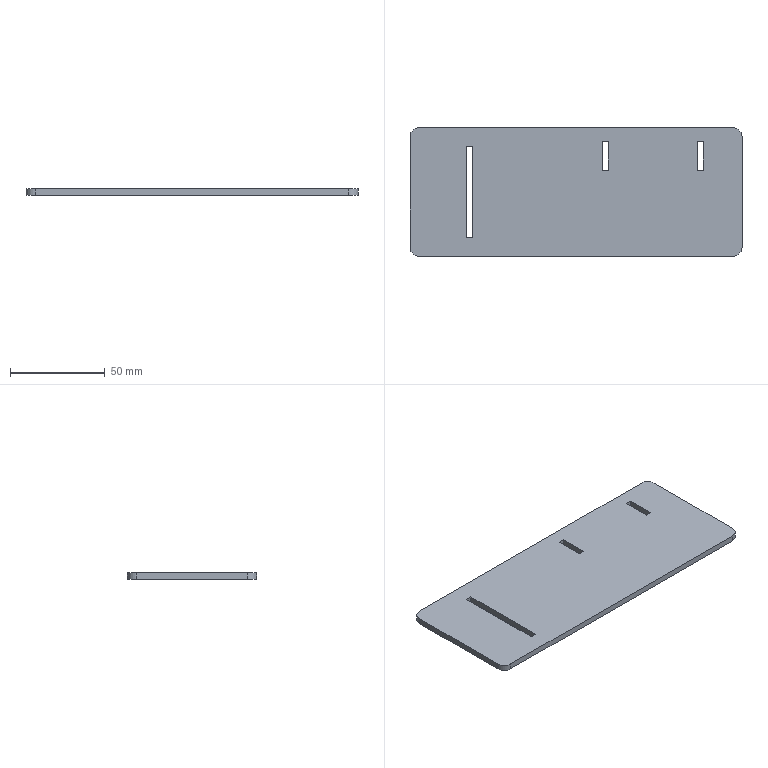Part | SolidWorks | features FlatPattern 1, SMBaseFlange 1, SheetMetal 1 | 1 solid | 22 faces | box 175 x 68 x 3.2 mm | volume 37213 mm3 | plane 18 | cylinder 4 | commonest cylinder face diameters 10 x4
STEP:
#1=CARTESIAN_POINT('',(-211.3,93.,3.2));
#2=VERTEX_POINT('',#1);
#3=CARTESIAN_POINT('',(-211.3,108.,3.2));
#4=VERTEX_POINT('',#3);
#5=CARTESIAN_POINT('',(-211.3,108.,3.2));
#6=DIRECTION('',(0.,1.,0.));
#7=VECTOR('',#6,1000.);
#8=LINE('',#5,#7);
#9=EDGE_CURVE('',#2,#4,#8,.T.);
#10=ORIENTED_EDGE('',*,*,#9,.F.);
#11=CARTESIAN_POINT('',(-214.5,93.,3.2));
#12=VERTEX_POINT('',#11);
#13=CARTESIAN_POINT('',(-211.3,93.,3.2));
#14=DIRECTION('',(1.,0.,0.));
#15=VECTOR('',#14,1000.);
#16=LINE('',#13,#15);
#17=EDGE_CURVE('',#12,#2,#16,.T.);
#18=ORIENTED_EDGE('',*,*,#17,.F.);
#19=CARTESIAN_POINT('',(-214.5,108.,3.2));
#20=VERTEX_POINT('',#19);
#21=CARTESIAN_POINT('',(-214.5,108.,3.2));
#22=DIRECTION('',(0.,-1.,0.));
#23=VECTOR('',#22,1000.);
#24=LINE('',#21,#23);
#25=EDGE_CURVE('',#20,#12,#24,.T.);
#26=ORIENTED_EDGE('',*,*,#25,.F.);
#27=CARTESIAN_POINT('',(-211.3,108.,3.2));
#28=DIRECTION('',(-1.,0.,0.));
#29=VECTOR('',#28,1000.);
#30=LINE('',#27,#29);
#31=EDGE_CURVE('',#4,#20,#30,.T.);
#32=ORIENTED_EDGE('',*,*,#31,.F.);
#33=EDGE_LOOP('',(#10,#18,#26,#32));
#34=FACE_BOUND('',#33,.T.);
#35=CARTESIAN_POINT('',(-190.9,110.5,3.2));
#36=VERTEX_POINT('',#35);
#37=CARTESIAN_POINT('',(-195.9,115.5,3.2));
#38=VERTEX_POINT('',#37);
#39=CARTESIAN_POINT('',(-195.9,110.5,3.2));
#40=DIRECTION('',(0.,0.,1.));
#41=DIRECTION('',(-1.,0.,0.));
#42=AXIS2_PLACEMENT_3D('',#39,#40,#41);
#43=CIRCLE('',#42,5.);
#44=EDGE_CURVE('',#36,#38,#43,.T.);
#45=ORIENTED_EDGE('',*,*,#44,.T.);
#46=CARTESIAN_POINT('',(-360.9,115.5,3.2));
#47=VERTEX_POINT('',#46);
#48=CARTESIAN_POINT('',(-360.9,115.5,3.2));
#49=DIRECTION('',(-1.,0.,0.));
#50=VECTOR('',#49,1000.);
#51=LINE('',#48,#50);
#52=EDGE_CURVE('',#38,#47,#51,.T.);
#53=ORIENTED_EDGE('',*,*,#52,.T.);
#54=CARTESIAN_POINT('',(-365.9,110.5,3.2));
#55=VERTEX_POINT('',#54);
#56=CARTESIAN_POINT('',(-360.9,110.5,3.2));
#57=DIRECTION('',(0.,0.,1.));
#58=DIRECTION('',(-1.,0.,0.));
#59=AXIS2_PLACEMENT_3D('',#56,#57,#58);
#60=CIRCLE('',#59,5.);
#61=EDGE_CURVE('',#47,#55,#60,.T.);
#62=ORIENTED_EDGE('',*,*,#61,.T.);
#63=CARTESIAN_POINT('',(-365.9,52.5,3.2));
#64=VERTEX_POINT('',#63);
#65=CARTESIAN_POINT('',(-365.9,52.5,3.2));
#66=DIRECTION('',(0.,-1.,0.));
#67=VECTOR('',#66,1000.);
#68=LINE('',#65,#67);
#69=EDGE_CURVE('',#55,#64,#68,.T.);
#70=ORIENTED_EDGE('',*,*,#69,.T.);
#71=CARTESIAN_POINT('',(-360.9,47.5,3.2));
#72=VERTEX_POINT('',#71);
#73=CARTESIAN_POINT('',(-360.9,52.5,3.2));
#74=DIRECTION('',(0.,0.,1.));
#75=DIRECTION('',(-1.,0.,0.));
#76=AXIS2_PLACEMENT_3D('',#73,#74,#75);
#77=CIRCLE('',#76,5.);
#78=EDGE_CURVE('',#64,#72,#77,.T.);
#79=ORIENTED_EDGE('',*,*,#78,.T.);
#80=CARTESIAN_POINT('',(-195.9,47.5,3.2));
#81=VERTEX_POINT('',#80);
#82=CARTESIAN_POINT('',(-360.9,47.5,3.2));
#83=DIRECTION('',(1.,0.,0.));
#84=VECTOR('',#83,1000.);
#85=LINE('',#82,#84);
#86=EDGE_CURVE('',#72,#81,#85,.T.);
#87=ORIENTED_EDGE('',*,*,#86,.T.);
#88=CARTESIAN_POINT('',(-190.9,52.5,3.2));
#89=VERTEX_POINT('',#88);
#90=CARTESIAN_POINT('',(-195.9,52.5,3.2));
#91=DIRECTION('',(0.,0.,1.));
#92=DIRECTION('',(1.,0.,0.));
#93=AXIS2_PLACEMENT_3D('',#90,#91,#92);
#94=CIRCLE('',#93,5.);
#95=EDGE_CURVE('',#81,#89,#94,.T.);
#96=ORIENTED_EDGE('',*,*,#95,.T.);
#97=CARTESIAN_POINT('',(-190.9,52.5,3.2));
#98=DIRECTION('',(0.,1.,0.));
#99=VECTOR('',#98,1000.);
#100=LINE('',#97,#99);
#101=EDGE_CURVE('',#89,#36,#100,.T.);
#102=ORIENTED_EDGE('',*,*,#101,.T.);
#103=EDGE_LOOP('',(#45,#53,#62,#70,#79,#87,#96,#102));
#104=FACE_OUTER_BOUND('',#103,.T.);
#105=CARTESIAN_POINT('',(-335.9,105.5,3.2));
#106=VERTEX_POINT('',#105);
#107=CARTESIAN_POINT('',(-335.9,57.5,3.2));
#108=VERTEX_POINT('',#107);
#109=CARTESIAN_POINT('',(-335.9,105.5,3.2));
#110=DIRECTION('',(0.,-1.,0.));
#111=VECTOR('',#110,1000.);
#112=LINE('',#109,#111);
#113=EDGE_CURVE('',#106,#108,#112,.T.);
#114=ORIENTED_EDGE('',*,*,#113,.F.);
#115=CARTESIAN_POINT('',(-332.7,105.5,3.2));
#116=VERTEX_POINT('',#115);
#117=CARTESIAN_POINT('',(-335.9,105.5,3.2));
#118=DIRECTION('',(-1.,0.,0.));
#119=VECTOR('',#118,1000.);
#120=LINE('',#117,#119);
#121=EDGE_CURVE('',#116,#106,#120,.T.);
#122=ORIENTED_EDGE('',*,*,#121,.F.);
#123=CARTESIAN_POINT('',(-332.7,57.5,3.2));
#124=VERTEX_POINT('',#123);
#125=CARTESIAN_POINT('',(-332.7,105.5,3.2));
#126=DIRECTION('',(0.,1.,0.));
#127=VECTOR('',#126,1000.);
#128=LINE('',#125,#127);
#129=EDGE_CURVE('',#124,#116,#128,.T.);
#130=ORIENTED_EDGE('',*,*,#129,.F.);
#131=CARTESIAN_POINT('',(-335.9,57.5,3.2));
#132=DIRECTION('',(1.,0.,0.));
#133=VECTOR('',#132,1000.);
#134=LINE('',#131,#133);
#135=EDGE_CURVE('',#108,#124,#134,.T.);
#136=ORIENTED_EDGE('',*,*,#135,.F.);
#137=EDGE_LOOP('',(#114,#122,#130,#136));
#138=FACE_BOUND('',#137,.T.);
#139=CARTESIAN_POINT('',(-261.3,93.,3.2));
#140=VERTEX_POINT('',#139);
#141=CARTESIAN_POINT('',(-261.3,108.,3.2));
#142=VERTEX_POINT('',#141);
#143=CARTESIAN_POINT('',(-261.3,108.,3.2));
#144=DIRECTION('',(0.,1.,0.));
#145=VECTOR('',#144,1000.);
#146=LINE('',#143,#145);
#147=EDGE_CURVE('',#140,#142,#146,.T.);
#148=ORIENTED_EDGE('',*,*,#147,.F.);
#149=CARTESIAN_POINT('',(-264.5,93.,3.2));
#150=VERTEX_POINT('',#149);
#151=CARTESIAN_POINT('',(-261.3,93.,3.2));
#152=DIRECTION('',(1.,0.,0.));
#153=VECTOR('',#152,1000.);
#154=LINE('',#151,#153);
#155=EDGE_CURVE('',#150,#140,#154,.T.);
#156=ORIENTED_EDGE('',*,*,#155,.F.);
#157=CARTESIAN_POINT('',(-264.5,108.,3.2));
#158=VERTEX_POINT('',#157);
#159=CARTESIAN_POINT('',(-264.5,108.,3.2));
#160=DIRECTION('',(0.,-1.,0.));
#161=VECTOR('',#160,1000.);
#162=LINE('',#159,#161);
#163=EDGE_CURVE('',#158,#150,#162,.T.);
#164=ORIENTED_EDGE('',*,*,#163,.F.);
#165=CARTESIAN_POINT('',(-261.3,108.,3.2));
#166=DIRECTION('',(-1.,0.,0.));
#167=VECTOR('',#166,1000.);
#168=LINE('',#165,#167);
#169=EDGE_CURVE('',#142,#158,#168,.T.);
#170=ORIENTED_EDGE('',*,*,#169,.F.);
#171=EDGE_LOOP('',(#148,#156,#164,#170));
#172=FACE_BOUND('',#171,.T.);
#173=CARTESIAN_POINT('',(-195.9,110.5,3.2));
#174=DIRECTION('',(0.,0.,-1.));
#175=DIRECTION('',(-1.,0.,0.));
#176=AXIS2_PLACEMENT_3D('',#173,#174,#175);
#177=PLANE('',#176);
#178=ADVANCED_FACE('',(#34,#104,#138,#172),#177,.F.);
#179=CARTESIAN_POINT('',(-190.9,110.5,0.));
#180=VERTEX_POINT('',#179);
#181=CARTESIAN_POINT('',(-195.9,115.5,0.));
#182=VERTEX_POINT('',#181);
#183=CARTESIAN_POINT('',(-195.9,110.5,0.));
#184=DIRECTION('',(0.,0.,1.));
#185=DIRECTION('',(-1.,0.,0.));
#186=AXIS2_PLACEMENT_3D('',#183,#184,#185);
#187=CIRCLE('',#186,5.);
#188=EDGE_CURVE('',#180,#182,#187,.T.);
#189=ORIENTED_EDGE('',*,*,#188,.F.);
#190=CARTESIAN_POINT('',(-190.9,52.5,0.));
#191=VERTEX_POINT('',#190);
#192=CARTESIAN_POINT('',(-190.9,52.5,0.));
#193=DIRECTION('',(0.,1.,0.));
#194=VECTOR('',#193,1000.);
#195=LINE('',#192,#194);
#196=EDGE_CURVE('',#191,#180,#195,.T.);
#197=ORIENTED_EDGE('',*,*,#196,.F.);
#198=CARTESIAN_POINT('',(-195.9,47.5,0.));
#199=VERTEX_POINT('',#198);
#200=CARTESIAN_POINT('',(-195.9,52.5,0.));
#201=DIRECTION('',(0.,0.,1.));
#202=DIRECTION('',(1.,0.,0.));
#203=AXIS2_PLACEMENT_3D('',#200,#201,#202);
#204=CIRCLE('',#203,5.);
#205=EDGE_CURVE('',#199,#191,#204,.T.);
#206=ORIENTED_EDGE('',*,*,#205,.F.);
#207=CARTESIAN_POINT('',(-360.9,47.5,0.));
#208=VERTEX_POINT('',#207);
#209=CARTESIAN_POINT('',(-360.9,47.5,0.));
#210=DIRECTION('',(1.,0.,0.));
#211=VECTOR('',#210,1000.);
#212=LINE('',#209,#211);
#213=EDGE_CURVE('',#208,#199,#212,.T.);
#214=ORIENTED_EDGE('',*,*,#213,.F.);
#215=CARTESIAN_POINT('',(-365.9,52.5,0.));
#216=VERTEX_POINT('',#215);
#217=CARTESIAN_POINT('',(-360.9,52.5,0.));
#218=DIRECTION('',(0.,0.,1.));
#219=DIRECTION('',(-1.,0.,0.));
#220=AXIS2_PLACEMENT_3D('',#217,#218,#219);
#221=CIRCLE('',#220,5.);
#222=EDGE_CURVE('',#216,#208,#221,.T.);
#223=ORIENTED_EDGE('',*,*,#222,.F.);
#224=CARTESIAN_POINT('',(-365.9,110.5,0.));
#225=VERTEX_POINT('',#224);
#226=CARTESIAN_POINT('',(-365.9,52.5,0.));
#227=DIRECTION('',(0.,-1.,0.));
#228=VECTOR('',#227,1000.);
#229=LINE('',#226,#228);
#230=EDGE_CURVE('',#225,#216,#229,.T.);
#231=ORIENTED_EDGE('',*,*,#230,.F.);
#232=CARTESIAN_POINT('',(-360.9,115.5,0.));
#233=VERTEX_POINT('',#232);
#234=CARTESIAN_POINT('',(-360.9,110.5,0.));
#235=DIRECTION('',(0.,0.,1.));
#236=DIRECTION('',(-1.,0.,0.));
#237=AXIS2_PLACEMENT_3D('',#234,#235,#236);
#238=CIRCLE('',#237,5.);
#239=EDGE_CURVE('',#233,#225,#238,.T.);
#240=ORIENTED_EDGE('',*,*,#239,.F.);
#241=CARTESIAN_POINT('',(-360.9,115.5,0.));
#242=DIRECTION('',(-1.,0.,0.));
#243=VECTOR('',#242,1000.);
#244=LINE('',#241,#243);
#245=EDGE_CURVE('',#182,#233,#244,.T.);
#246=ORIENTED_EDGE('',*,*,#245,.F.);
#247=EDGE_LOOP('',(#189,#197,#206,#214,#223,#231,#240,#246));
#248=FACE_OUTER_BOUND('',#247,.T.);
#249=CARTESIAN_POINT('',(-332.7,105.5,0.));
#250=VERTEX_POINT('',#249);
#251=CARTESIAN_POINT('',(-335.9,105.5,0.));
#252=VERTEX_POINT('',#251);
#253=CARTESIAN_POINT('',(-335.9,105.5,0.));
#254=DIRECTION('',(-1.,0.,0.));
#255=VECTOR('',#254,1000.);
#256=LINE('',#253,#255);
#257=EDGE_CURVE('',#250,#252,#256,.T.);
#258=ORIENTED_EDGE('',*,*,#257,.T.);
#259=CARTESIAN_POINT('',(-335.9,57.5,0.));
#260=VERTEX_POINT('',#259);
#261=CARTESIAN_POINT('',(-335.9,105.5,0.));
#262=DIRECTION('',(0.,-1.,0.));
#263=VECTOR('',#262,1000.);
#264=LINE('',#261,#263);
#265=EDGE_CURVE('',#252,#260,#264,.T.);
#266=ORIENTED_EDGE('',*,*,#265,.T.);
#267=CARTESIAN_POINT('',(-332.7,57.5,0.));
#268=VERTEX_POINT('',#267);
#269=CARTESIAN_POINT('',(-335.9,57.5,0.));
#270=DIRECTION('',(1.,0.,0.));
#271=VECTOR('',#270,1000.);
#272=LINE('',#269,#271);
#273=EDGE_CURVE('',#260,#268,#272,.T.);
#274=ORIENTED_EDGE('',*,*,#273,.T.);
#275=CARTESIAN_POINT('',(-332.7,105.5,0.));
#276=DIRECTION('',(0.,1.,0.));
#277=VECTOR('',#276,1000.);
#278=LINE('',#275,#277);
#279=EDGE_CURVE('',#268,#250,#278,.T.);
#280=ORIENTED_EDGE('',*,*,#279,.T.);
#281=EDGE_LOOP('',(#258,#266,#274,#280));
#282=FACE_BOUND('',#281,.T.);
#283=CARTESIAN_POINT('',(-214.5,93.,0.));
#284=VERTEX_POINT('',#283);
#285=CARTESIAN_POINT('',(-211.3,93.,0.));
#286=VERTEX_POINT('',#285);
#287=CARTESIAN_POINT('',(-211.3,93.,0.));
#288=DIRECTION('',(1.,0.,0.));
#289=VECTOR('',#288,1000.);
#290=LINE('',#287,#289);
#291=EDGE_CURVE('',#284,#286,#290,.T.);
#292=ORIENTED_EDGE('',*,*,#291,.T.);
#293=CARTESIAN_POINT('',(-211.3,108.,0.));
#294=VERTEX_POINT('',#293);
#295=CARTESIAN_POINT('',(-211.3,108.,0.));
#296=DIRECTION('',(0.,1.,0.));
#297=VECTOR('',#296,1000.);
#298=LINE('',#295,#297);
#299=EDGE_CURVE('',#286,#294,#298,.T.);
#300=ORIENTED_EDGE('',*,*,#299,.T.);
#301=CARTESIAN_POINT('',(-214.5,108.,0.));
#302=VERTEX_POINT('',#301);
#303=CARTESIAN_POINT('',(-211.3,108.,0.));
#304=DIRECTION('',(-1.,0.,0.));
#305=VECTOR('',#304,1000.);
#306=LINE('',#303,#305);
#307=EDGE_CURVE('',#294,#302,#306,.T.);
#308=ORIENTED_EDGE('',*,*,#307,.T.);
#309=CARTESIAN_POINT('',(-214.5,108.,0.));
#310=DIRECTION('',(0.,-1.,0.));
#311=VECTOR('',#310,1000.);
#312=LINE('',#309,#311);
#313=EDGE_CURVE('',#302,#284,#312,.T.);
#314=ORIENTED_EDGE('',*,*,#313,.T.);
#315=EDGE_LOOP('',(#292,#300,#308,#314));
#316=FACE_BOUND('',#315,.T.);
#317=CARTESIAN_POINT('',(-264.5,93.,0.));
#318=VERTEX_POINT('',#317);
#319=CARTESIAN_POINT('',(-261.3,93.,0.));
#320=VERTEX_POINT('',#319);
#321=CARTESIAN_POINT('',(-261.3,93.,0.));
#322=DIRECTION('',(1.,0.,0.));
#323=VECTOR('',#322,1000.);
#324=LINE('',#321,#323);
#325=EDGE_CURVE('',#318,#320,#324,.T.);
#326=ORIENTED_EDGE('',*,*,#325,.T.);
#327=CARTESIAN_POINT('',(-261.3,108.,0.));
#328=VERTEX_POINT('',#327);
#329=CARTESIAN_POINT('',(-261.3,108.,0.));
#330=DIRECTION('',(0.,1.,0.));
#331=VECTOR('',#330,1000.);
#332=LINE('',#329,#331);
#333=EDGE_CURVE('',#320,#328,#332,.T.);
#334=ORIENTED_EDGE('',*,*,#333,.T.);
#335=CARTESIAN_POINT('',(-264.5,108.,0.));
#336=VERTEX_POINT('',#335);
#337=CARTESIAN_POINT('',(-261.3,108.,0.));
#338=DIRECTION('',(-1.,0.,0.));
#339=VECTOR('',#338,1000.);
#340=LINE('',#337,#339);
#341=EDGE_CURVE('',#328,#336,#340,.T.);
#342=ORIENTED_EDGE('',*,*,#341,.T.);
#343=CARTESIAN_POINT('',(-264.5,108.,0.));
#344=DIRECTION('',(0.,-1.,0.));
#345=VECTOR('',#344,1000.);
#346=LINE('',#343,#345);
#347=EDGE_CURVE('',#336,#318,#346,.T.);
#348=ORIENTED_EDGE('',*,*,#347,.T.);
#349=EDGE_LOOP('',(#326,#334,#342,#348));
#350=FACE_BOUND('',#349,.T.);
#351=CARTESIAN_POINT('',(-195.9,110.5,0.));
#352=DIRECTION('',(0.,0.,-1.));
#353=DIRECTION('',(-1.,0.,0.));
#354=AXIS2_PLACEMENT_3D('',#351,#352,#353);
#355=PLANE('',#354);
#356=ADVANCED_FACE('',(#248,#282,#316,#350),#355,.T.);
#357=ORIENTED_EDGE('',*,*,#188,.T.);
#358=CARTESIAN_POINT('',(-195.9,115.5,3.2));
#359=DIRECTION('',(0.,0.,-1.));
#360=VECTOR('',#359,1000.);
#361=LINE('',#358,#360);
#362=EDGE_CURVE('',#38,#182,#361,.T.);
#363=ORIENTED_EDGE('',*,*,#362,.F.);
#364=ORIENTED_EDGE('',*,*,#44,.F.);
#365=CARTESIAN_POINT('',(-190.9,110.5,3.2));
#366=DIRECTION('',(0.,0.,-1.));
#367=VECTOR('',#366,1000.);
#368=LINE('',#365,#367);
#369=EDGE_CURVE('',#36,#180,#368,.T.);
#370=ORIENTED_EDGE('',*,*,#369,.T.);
#371=EDGE_LOOP('',(#357,#363,#364,#370));
#372=FACE_OUTER_BOUND('',#371,.T.);
#373=CARTESIAN_POINT('',(-195.9,110.5,3.2));
#374=DIRECTION('',(0.,0.,-1.));
#375=DIRECTION('',(-1.,0.,0.));
#376=AXIS2_PLACEMENT_3D('',#373,#374,#375);
#377=CYLINDRICAL_SURFACE('',#376,5.);
#378=ADVANCED_FACE('',(#372),#377,.T.);
#379=ORIENTED_EDGE('',*,*,#245,.T.);
#380=CARTESIAN_POINT('',(-360.9,115.5,3.2));
#381=DIRECTION('',(0.,0.,-1.));
#382=VECTOR('',#381,1000.);
#383=LINE('',#380,#382);
#384=EDGE_CURVE('',#47,#233,#383,.T.);
#385=ORIENTED_EDGE('',*,*,#384,.F.);
#386=ORIENTED_EDGE('',*,*,#52,.F.);
#387=ORIENTED_EDGE('',*,*,#362,.T.);
#388=EDGE_LOOP('',(#379,#385,#386,#387));
#389=FACE_OUTER_BOUND('',#388,.T.);
#390=CARTESIAN_POINT('',(-360.9,115.5,3.2));
#391=DIRECTION('',(0.,-1.,0.));
#392=DIRECTION('',(0.,0.,-1.));
#393=AXIS2_PLACEMENT_3D('',#390,#391,#392);
#394=PLANE('',#393);
#395=ADVANCED_FACE('',(#389),#394,.F.);
#396=ORIENTED_EDGE('',*,*,#239,.T.);
#397=CARTESIAN_POINT('',(-365.9,110.5,3.2));
#398=DIRECTION('',(0.,0.,-1.));
#399=VECTOR('',#398,1000.);
#400=LINE('',#397,#399);
#401=EDGE_CURVE('',#55,#225,#400,.T.);
#402=ORIENTED_EDGE('',*,*,#401,.F.);
#403=ORIENTED_EDGE('',*,*,#61,.F.);
#404=ORIENTED_EDGE('',*,*,#384,.T.);
#405=EDGE_LOOP('',(#396,#402,#403,#404));
#406=FACE_OUTER_BOUND('',#405,.T.);
#407=CARTESIAN_POINT('',(-360.9,110.5,3.2));
#408=DIRECTION('',(0.,0.,-1.));
#409=DIRECTION('',(-1.,0.,0.));
#410=AXIS2_PLACEMENT_3D('',#407,#408,#409);
#411=CYLINDRICAL_SURFACE('',#410,5.);
#412=ADVANCED_FACE('',(#406),#411,.T.);
#413=ORIENTED_EDGE('',*,*,#230,.T.);
#414=CARTESIAN_POINT('',(-365.9,52.5,3.2));
#415=DIRECTION('',(0.,0.,-1.));
#416=VECTOR('',#415,1000.);
#417=LINE('',#414,#416);
#418=EDGE_CURVE('',#64,#216,#417,.T.);
#419=ORIENTED_EDGE('',*,*,#418,.F.);
#420=ORIENTED_EDGE('',*,*,#69,.F.);
#421=ORIENTED_EDGE('',*,*,#401,.T.);
#422=EDGE_LOOP('',(#413,#419,#420,#421));
#423=FACE_OUTER_BOUND('',#422,.T.);
#424=CARTESIAN_POINT('',(-365.9,52.5,3.2));
#425=DIRECTION('',(1.,0.,0.));
#426=DIRECTION('',(0.,0.,-1.));
#427=AXIS2_PLACEMENT_3D('',#424,#425,#426);
#428=PLANE('',#427);
#429=ADVANCED_FACE('',(#423),#428,.F.);
#430=ORIENTED_EDGE('',*,*,#222,.T.);
#431=CARTESIAN_POINT('',(-360.9,47.5,3.2));
#432=DIRECTION('',(0.,0.,-1.));
#433=VECTOR('',#432,1000.);
#434=LINE('',#431,#433);
#435=EDGE_CURVE('',#72,#208,#434,.T.);
#436=ORIENTED_EDGE('',*,*,#435,.F.);
#437=ORIENTED_EDGE('',*,*,#78,.F.);
#438=ORIENTED_EDGE('',*,*,#418,.T.);
#439=EDGE_LOOP('',(#430,#436,#437,#438));
#440=FACE_OUTER_BOUND('',#439,.T.);
#441=CARTESIAN_POINT('',(-360.9,52.5,3.2));
#442=DIRECTION('',(0.,0.,-1.));
#443=DIRECTION('',(-1.,0.,0.));
#444=AXIS2_PLACEMENT_3D('',#441,#442,#443);
#445=CYLINDRICAL_SURFACE('',#444,5.);
#446=ADVANCED_FACE('',(#440),#445,.T.);
#447=ORIENTED_EDGE('',*,*,#213,.T.);
#448=CARTESIAN_POINT('',(-195.9,47.5,3.2));
#449=DIRECTION('',(0.,0.,-1.));
#450=VECTOR('',#449,1000.);
#451=LINE('',#448,#450);
#452=EDGE_CURVE('',#81,#199,#451,.T.);
#453=ORIENTED_EDGE('',*,*,#452,.F.);
#454=ORIENTED_EDGE('',*,*,#86,.F.);
#455=ORIENTED_EDGE('',*,*,#435,.T.);
#456=EDGE_LOOP('',(#447,#453,#454,#455));
#457=FACE_OUTER_BOUND('',#456,.T.);
#458=CARTESIAN_POINT('',(-360.9,47.5,3.2));
#459=DIRECTION('',(0.,1.,0.));
#460=DIRECTION('',(0.,0.,1.));
#461=AXIS2_PLACEMENT_3D('',#458,#459,#460);
#462=PLANE('',#461);
#463=ADVANCED_FACE('',(#457),#462,.F.);
#464=ORIENTED_EDGE('',*,*,#205,.T.);
#465=CARTESIAN_POINT('',(-190.9,52.5,3.2));
#466=DIRECTION('',(0.,0.,-1.));
#467=VECTOR('',#466,1000.);
#468=LINE('',#465,#467);
#469=EDGE_CURVE('',#89,#191,#468,.T.);
#470=ORIENTED_EDGE('',*,*,#469,.F.);
#471=ORIENTED_EDGE('',*,*,#95,.F.);
#472=ORIENTED_EDGE('',*,*,#452,.T.);
#473=EDGE_LOOP('',(#464,#470,#471,#472));
#474=FACE_OUTER_BOUND('',#473,.T.);
#475=CARTESIAN_POINT('',(-195.9,52.5,3.2));
#476=DIRECTION('',(0.,0.,-1.));
#477=DIRECTION('',(-1.,0.,0.));
#478=AXIS2_PLACEMENT_3D('',#475,#476,#477);
#479=CYLINDRICAL_SURFACE('',#478,5.);
#480=ADVANCED_FACE('',(#474),#479,.T.);
#481=ORIENTED_EDGE('',*,*,#196,.T.);
#482=ORIENTED_EDGE('',*,*,#369,.F.);
#483=ORIENTED_EDGE('',*,*,#101,.F.);
#484=ORIENTED_EDGE('',*,*,#469,.T.);
#485=EDGE_LOOP('',(#481,#482,#483,#484));
#486=FACE_OUTER_BOUND('',#485,.T.);
#487=CARTESIAN_POINT('',(-190.9,52.5,3.2));
#488=DIRECTION('',(-1.,0.,0.));
#489=DIRECTION('',(0.,0.,1.));
#490=AXIS2_PLACEMENT_3D('',#487,#488,#489);
#491=PLANE('',#490);
#492=ADVANCED_FACE('',(#486),#491,.F.);
#493=ORIENTED_EDGE('',*,*,#265,.F.);
#494=CARTESIAN_POINT('',(-335.9,105.5,3.2));
#495=DIRECTION('',(0.,0.,-1.));
#496=VECTOR('',#495,1000.);
#497=LINE('',#494,#496);
#498=EDGE_CURVE('',#106,#252,#497,.T.);
#499=ORIENTED_EDGE('',*,*,#498,.F.);
#500=ORIENTED_EDGE('',*,*,#113,.T.);
#501=CARTESIAN_POINT('',(-335.9,57.5,3.2));
#502=DIRECTION('',(0.,0.,-1.));
#503=VECTOR('',#502,1000.);
#504=LINE('',#501,#503);
#505=EDGE_CURVE('',#108,#260,#504,.T.);
#506=ORIENTED_EDGE('',*,*,#505,.T.);
#507=EDGE_LOOP('',(#493,#499,#500,#506));
#508=FACE_OUTER_BOUND('',#507,.T.);
#509=CARTESIAN_POINT('',(-335.9,105.5,3.2));
#510=DIRECTION('',(1.,0.,0.));
#511=DIRECTION('',(0.,0.,-1.));
#512=AXIS2_PLACEMENT_3D('',#509,#510,#511);
#513=PLANE('',#512);
#514=ADVANCED_FACE('',(#508),#513,.T.);
#515=ORIENTED_EDGE('',*,*,#273,.F.);
#516=ORIENTED_EDGE('',*,*,#505,.F.);
#517=ORIENTED_EDGE('',*,*,#135,.T.);
#518=CARTESIAN_POINT('',(-332.7,57.5,3.2));
#519=DIRECTION('',(0.,0.,-1.));
#520=VECTOR('',#519,1000.);
#521=LINE('',#518,#520);
#522=EDGE_CURVE('',#124,#268,#521,.T.);
#523=ORIENTED_EDGE('',*,*,#522,.T.);
#524=EDGE_LOOP('',(#515,#516,#517,#523));
#525=FACE_OUTER_BOUND('',#524,.T.);
#526=CARTESIAN_POINT('',(-335.9,57.5,3.2));
#527=DIRECTION('',(0.,1.,0.));
#528=DIRECTION('',(0.,0.,1.));
#529=AXIS2_PLACEMENT_3D('',#526,#527,#528);
#530=PLANE('',#529);
#531=ADVANCED_FACE('',(#525),#530,.T.);
#532=ORIENTED_EDGE('',*,*,#279,.F.);
#533=ORIENTED_EDGE('',*,*,#522,.F.);
#534=ORIENTED_EDGE('',*,*,#129,.T.);
#535=CARTESIAN_POINT('',(-332.7,105.5,3.2));
#536=DIRECTION('',(0.,0.,-1.));
#537=VECTOR('',#536,1000.);
#538=LINE('',#535,#537);
#539=EDGE_CURVE('',#116,#250,#538,.T.);
#540=ORIENTED_EDGE('',*,*,#539,.T.);
#541=EDGE_LOOP('',(#532,#533,#534,#540));
#542=FACE_OUTER_BOUND('',#541,.T.);
#543=CARTESIAN_POINT('',(-332.7,105.5,3.2));
#544=DIRECTION('',(-1.,0.,0.));
#545=DIRECTION('',(0.,0.,1.));
#546=AXIS2_PLACEMENT_3D('',#543,#544,#545);
#547=PLANE('',#546);
#548=ADVANCED_FACE('',(#542),#547,.T.);
#549=ORIENTED_EDGE('',*,*,#257,.F.);
#550=ORIENTED_EDGE('',*,*,#539,.F.);
#551=ORIENTED_EDGE('',*,*,#121,.T.);
#552=ORIENTED_EDGE('',*,*,#498,.T.);
#553=EDGE_LOOP('',(#549,#550,#551,#552));
#554=FACE_OUTER_BOUND('',#553,.T.);
#555=CARTESIAN_POINT('',(-335.9,105.5,3.2));
#556=DIRECTION('',(0.,-1.,0.));
#557=DIRECTION('',(0.,0.,-1.));
#558=AXIS2_PLACEMENT_3D('',#555,#556,#557);
#559=PLANE('',#558);
#560=ADVANCED_FACE('',(#554),#559,.T.);
#561=ORIENTED_EDGE('',*,*,#299,.F.);
#562=CARTESIAN_POINT('',(-211.3,93.,3.2));
#563=DIRECTION('',(0.,0.,-1.));
#564=VECTOR('',#563,1000.);
#565=LINE('',#562,#564);
#566=EDGE_CURVE('',#2,#286,#565,.T.);
#567=ORIENTED_EDGE('',*,*,#566,.F.);
#568=ORIENTED_EDGE('',*,*,#9,.T.);
#569=CARTESIAN_POINT('',(-211.3,108.,3.2));
#570=DIRECTION('',(0.,0.,-1.));
#571=VECTOR('',#570,1000.);
#572=LINE('',#569,#571);
#573=EDGE_CURVE('',#4,#294,#572,.T.);
#574=ORIENTED_EDGE('',*,*,#573,.T.);
#575=EDGE_LOOP('',(#561,#567,#568,#574));
#576=FACE_OUTER_BOUND('',#575,.T.);
#577=CARTESIAN_POINT('',(-211.3,108.,3.2));
#578=DIRECTION('',(-1.,0.,0.));
#579=DIRECTION('',(0.,0.,1.));
#580=AXIS2_PLACEMENT_3D('',#577,#578,#579);
#581=PLANE('',#580);
#582=ADVANCED_FACE('',(#576),#581,.T.);
#583=ORIENTED_EDGE('',*,*,#307,.F.);
#584=ORIENTED_EDGE('',*,*,#573,.F.);
#585=ORIENTED_EDGE('',*,*,#31,.T.);
#586=CARTESIAN_POINT('',(-214.5,108.,3.2));
#587=DIRECTION('',(0.,0.,-1.));
#588=VECTOR('',#587,1000.);
#589=LINE('',#586,#588);
#590=EDGE_CURVE('',#20,#302,#589,.T.);
#591=ORIENTED_EDGE('',*,*,#590,.T.);
#592=EDGE_LOOP('',(#583,#584,#585,#591));
#593=FACE_OUTER_BOUND('',#592,.T.);
#594=CARTESIAN_POINT('',(-211.3,108.,3.2));
#595=DIRECTION('',(0.,-1.,0.));
#596=DIRECTION('',(0.,0.,-1.));
#597=AXIS2_PLACEMENT_3D('',#594,#595,#596);
#598=PLANE('',#597);
#599=ADVANCED_FACE('',(#593),#598,.T.);
#600=ORIENTED_EDGE('',*,*,#313,.F.);
#601=ORIENTED_EDGE('',*,*,#590,.F.);
#602=ORIENTED_EDGE('',*,*,#25,.T.);
#603=CARTESIAN_POINT('',(-214.5,93.,3.2));
#604=DIRECTION('',(0.,0.,-1.));
#605=VECTOR('',#604,1000.);
#606=LINE('',#603,#605);
#607=EDGE_CURVE('',#12,#284,#606,.T.);
#608=ORIENTED_EDGE('',*,*,#607,.T.);
#609=EDGE_LOOP('',(#600,#601,#602,#608));
#610=FACE_OUTER_BOUND('',#609,.T.);
#611=CARTESIAN_POINT('',(-214.5,108.,3.2));
#612=DIRECTION('',(1.,0.,0.));
#613=DIRECTION('',(0.,0.,-1.));
#614=AXIS2_PLACEMENT_3D('',#611,#612,#613);
#615=PLANE('',#614);
#616=ADVANCED_FACE('',(#610),#615,.T.);
#617=ORIENTED_EDGE('',*,*,#291,.F.);
#618=ORIENTED_EDGE('',*,*,#607,.F.);
#619=ORIENTED_EDGE('',*,*,#17,.T.);
#620=ORIENTED_EDGE('',*,*,#566,.T.);
#621=EDGE_LOOP('',(#617,#618,#619,#620));
#622=FACE_OUTER_BOUND('',#621,.T.);
#623=CARTESIAN_POINT('',(-211.3,93.,3.2));
#624=DIRECTION('',(0.,1.,0.));
#625=DIRECTION('',(0.,0.,1.));
#626=AXIS2_PLACEMENT_3D('',#623,#624,#625);
#627=PLANE('',#626);
#628=ADVANCED_FACE('',(#622),#627,.T.);
#629=ORIENTED_EDGE('',*,*,#333,.F.);
#630=CARTESIAN_POINT('',(-261.3,93.,3.2));
#631=DIRECTION('',(0.,0.,-1.));
#632=VECTOR('',#631,1000.);
#633=LINE('',#630,#632);
#634=EDGE_CURVE('',#140,#320,#633,.T.);
#635=ORIENTED_EDGE('',*,*,#634,.F.);
#636=ORIENTED_EDGE('',*,*,#147,.T.);
#637=CARTESIAN_POINT('',(-261.3,108.,3.2));
#638=DIRECTION('',(0.,0.,-1.));
#639=VECTOR('',#638,1000.);
#640=LINE('',#637,#639);
#641=EDGE_CURVE('',#142,#328,#640,.T.);
#642=ORIENTED_EDGE('',*,*,#641,.T.);
#643=EDGE_LOOP('',(#629,#635,#636,#642));
#644=FACE_OUTER_BOUND('',#643,.T.);
#645=CARTESIAN_POINT('',(-261.3,108.,3.2));
#646=DIRECTION('',(-1.,0.,0.));
#647=DIRECTION('',(0.,0.,1.));
#648=AXIS2_PLACEMENT_3D('',#645,#646,#647);
#649=PLANE('',#648);
#650=ADVANCED_FACE('',(#644),#649,.T.);
#651=ORIENTED_EDGE('',*,*,#341,.F.);
#652=ORIENTED_EDGE('',*,*,#641,.F.);
#653=ORIENTED_EDGE('',*,*,#169,.T.);
#654=CARTESIAN_POINT('',(-264.5,108.,3.2));
#655=DIRECTION('',(0.,0.,-1.));
#656=VECTOR('',#655,1000.);
#657=LINE('',#654,#656);
#658=EDGE_CURVE('',#158,#336,#657,.T.);
#659=ORIENTED_EDGE('',*,*,#658,.T.);
#660=EDGE_LOOP('',(#651,#652,#653,#659));
#661=FACE_OUTER_BOUND('',#660,.T.);
#662=CARTESIAN_POINT('',(-261.3,108.,3.2));
#663=DIRECTION('',(0.,-1.,0.));
#664=DIRECTION('',(0.,0.,-1.));
#665=AXIS2_PLACEMENT_3D('',#662,#663,#664);
#666=PLANE('',#665);
#667=ADVANCED_FACE('',(#661),#666,.T.);
#668=ORIENTED_EDGE('',*,*,#347,.F.);
#669=ORIENTED_EDGE('',*,*,#658,.F.);
#670=ORIENTED_EDGE('',*,*,#163,.T.);
#671=CARTESIAN_POINT('',(-264.5,93.,3.2));
#672=DIRECTION('',(0.,0.,-1.));
#673=VECTOR('',#672,1000.);
#674=LINE('',#671,#673);
#675=EDGE_CURVE('',#150,#318,#674,.T.);
#676=ORIENTED_EDGE('',*,*,#675,.T.);
#677=EDGE_LOOP('',(#668,#669,#670,#676));
#678=FACE_OUTER_BOUND('',#677,.T.);
#679=CARTESIAN_POINT('',(-264.5,108.,3.2));
#680=DIRECTION('',(1.,0.,0.));
#681=DIRECTION('',(0.,0.,-1.));
#682=AXIS2_PLACEMENT_3D('',#679,#680,#681);
#683=PLANE('',#682);
#684=ADVANCED_FACE('',(#678),#683,.T.);
#685=ORIENTED_EDGE('',*,*,#325,.F.);
#686=ORIENTED_EDGE('',*,*,#675,.F.);
#687=ORIENTED_EDGE('',*,*,#155,.T.);
#688=ORIENTED_EDGE('',*,*,#634,.T.);
#689=EDGE_LOOP('',(#685,#686,#687,#688));
#690=FACE_OUTER_BOUND('',#689,.T.);
#691=CARTESIAN_POINT('',(-261.3,93.,3.2));
#692=DIRECTION('',(0.,1.,0.));
#693=DIRECTION('',(0.,0.,1.));
#694=AXIS2_PLACEMENT_3D('',#691,#692,#693);
#695=PLANE('',#694);
#696=ADVANCED_FACE('',(#690),#695,.T.);
#697=CLOSED_SHELL('',(#178,#356,#378,#395,#412,#429,#446,#463,#480,#492,#514,#531,#548,#560,#582,#599,#616,#628,#650,#667,#684,#696));
#698=MANIFOLD_SOLID_BREP('',#697);
#699=CARTESIAN_POINT('',(0.,0.,0.));
#700=DIRECTION('',(0.,0.,1.));
#701=DIRECTION('',(1.,0.,0.));
#702=AXIS2_PLACEMENT_3D('',#699,#700,#701);
#703=(LENGTH_UNIT()NAMED_UNIT(*)SI_UNIT(.MILLI.,.METRE.));
#704=UNCERTAINTY_MEASURE_WITH_UNIT(LENGTH_MEASURE(0.00001),#703,'','');
#705=(NAMED_UNIT(*)PLANE_ANGLE_UNIT()SI_UNIT($,.RADIAN.));
#706=(NAMED_UNIT(*)SI_UNIT($,.STERADIAN.)SOLID_ANGLE_UNIT());
#707=(GEOMETRIC_REPRESENTATION_CONTEXT(3)GLOBAL_UNCERTAINTY_ASSIGNED_CONTEXT((#704))GLOBAL_UNIT_ASSIGNED_CONTEXT((#703,#705,#706))REPRESENTATION_CONTEXT('',''));
#708=ADVANCED_BREP_SHAPE_REPRESENTATION('',(#698,#702),#707);